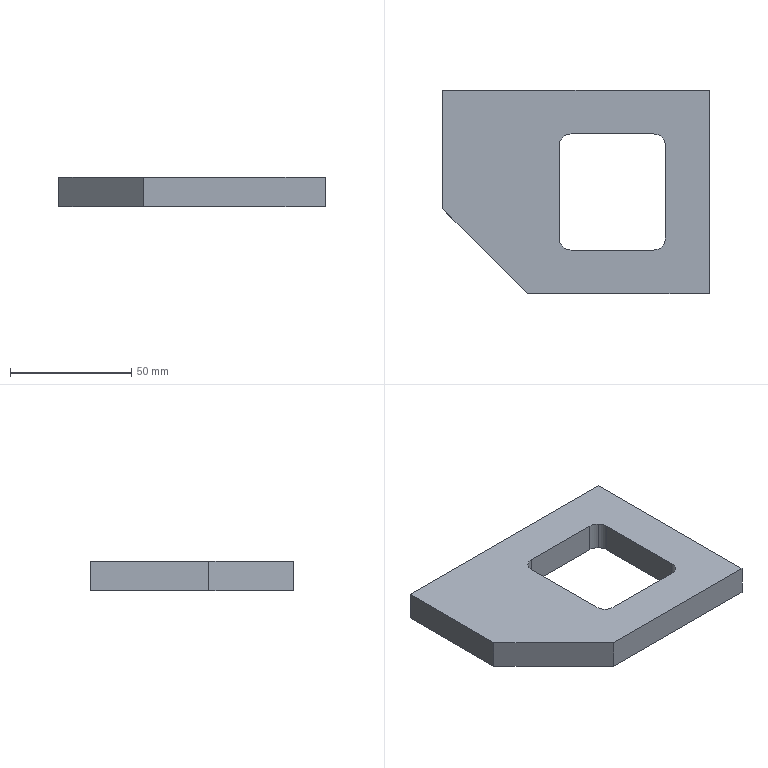Part | STEP file | ASND-0110-Body 1-28 | 1 solid | 19 faces | box 110 x 84 x 12 mm | volume 78444 mm3 | plane 11 | cylinder 8 | commonest cylinder face diameters 10 x8